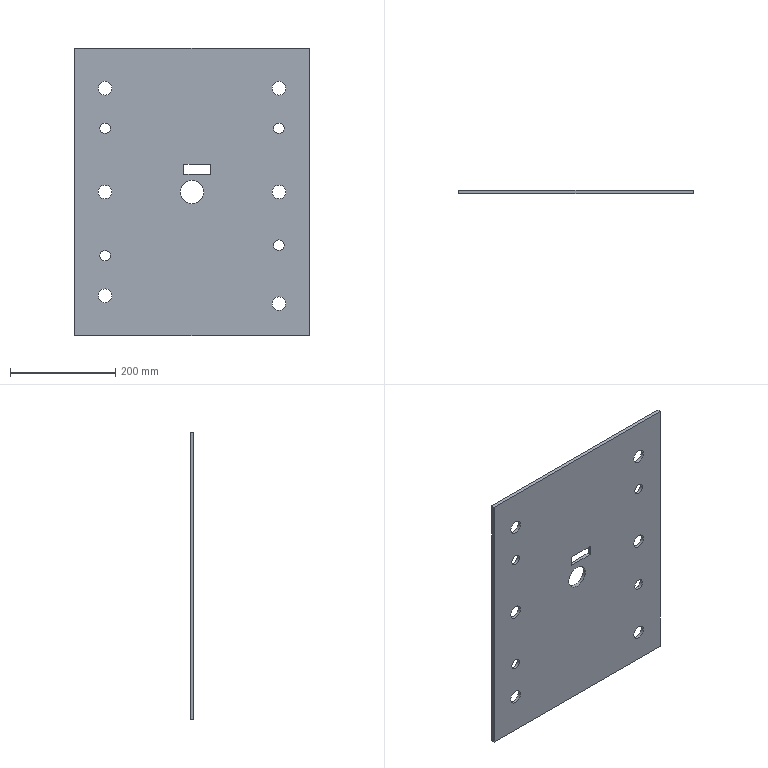Part | STEP file | INSULT-PLATE_id454_x_t | 1 solid | 21 faces | box 446 x 6 x 546 mm | volume 1419506 mm3 | cylinder 11 | plane 10 | commonest cylinder face diameters 26 x6 20 x4 44 x1
STEP:
#1=CARTESIAN_POINT('',(35.5,-296.5,34.));
#2=VERTEX_POINT('',#1);
#3=CARTESIAN_POINT('',(-15.5,-296.5,34.));
#4=VERTEX_POINT('',#3);
#5=CARTESIAN_POINT('',(-15.5,-296.5,34.));
#6=DIRECTION('',(-1.,0.,0.));
#7=VECTOR('',#6,1.);
#8=LINE('',#5,#7);
#9=EDGE_CURVE('',#2,#4,#8,.T.);
#10=ORIENTED_EDGE('',*,*,#9,.T.);
#11=CARTESIAN_POINT('',(-15.5,-296.5,53.));
#12=VERTEX_POINT('',#11);
#13=CARTESIAN_POINT('',(-15.5,-296.5,53.));
#14=DIRECTION('',(0.,0.,1.));
#15=VECTOR('',#14,1.);
#16=LINE('',#13,#15);
#17=EDGE_CURVE('',#4,#12,#16,.T.);
#18=ORIENTED_EDGE('',*,*,#17,.T.);
#19=CARTESIAN_POINT('',(35.5,-296.5,53.));
#20=VERTEX_POINT('',#19);
#21=CARTESIAN_POINT('',(35.5,-296.5,53.));
#22=DIRECTION('',(1.,0.,0.));
#23=VECTOR('',#22,1.);
#24=LINE('',#21,#23);
#25=EDGE_CURVE('',#12,#20,#24,.T.);
#26=ORIENTED_EDGE('',*,*,#25,.T.);
#27=CARTESIAN_POINT('',(35.5,-296.5,34.));
#28=DIRECTION('',(0.,0.,-1.));
#29=VECTOR('',#28,1.);
#30=LINE('',#27,#29);
#31=EDGE_CURVE('',#20,#2,#30,.T.);
#32=ORIENTED_EDGE('',*,*,#31,.T.);
#33=EDGE_LOOP('',(#10,#18,#26,#32));
#34=FACE_BOUND('',#33,.T.);
#35=CARTESIAN_POINT('',(165.,-296.5,-225.));
#36=VERTEX_POINT('',#35);
#37=CARTESIAN_POINT('',(165.,-296.5,-212.));
#38=DIRECTION('',(0.,1.,0.));
#39=DIRECTION('',(0.,0.,-1.));
#40=AXIS2_PLACEMENT_3D('',#37,#38,#39);
#41=CIRCLE('',#40,13.);
#42=EDGE_CURVE('',#36,#36,#41,.T.);
#43=ORIENTED_EDGE('',*,*,#42,.T.);
#44=EDGE_LOOP('',(#43));
#45=FACE_BOUND('',#44,.T.);
#46=CARTESIAN_POINT('',(165.,-296.5,-111.));
#47=VERTEX_POINT('',#46);
#48=CARTESIAN_POINT('',(165.,-296.5,-101.));
#49=DIRECTION('',(0.,1.,0.));
#50=DIRECTION('',(0.,0.,-1.));
#51=AXIS2_PLACEMENT_3D('',#48,#49,#50);
#52=CIRCLE('',#51,10.);
#53=EDGE_CURVE('',#47,#47,#52,.T.);
#54=ORIENTED_EDGE('',*,*,#53,.T.);
#55=EDGE_LOOP('',(#54));
#56=FACE_BOUND('',#55,.T.);
#57=CARTESIAN_POINT('',(165.,-296.5,-13.));
#58=VERTEX_POINT('',#57);
#59=CARTESIAN_POINT('',(165.,-296.5,0.));
#60=DIRECTION('',(0.,1.,0.));
#61=DIRECTION('',(0.,0.,-1.));
#62=AXIS2_PLACEMENT_3D('',#59,#60,#61);
#63=CIRCLE('',#62,13.);
#64=EDGE_CURVE('',#58,#58,#63,.T.);
#65=ORIENTED_EDGE('',*,*,#64,.T.);
#66=EDGE_LOOP('',(#65));
#67=FACE_BOUND('',#66,.T.);
#68=CARTESIAN_POINT('',(165.,-296.5,111.));
#69=VERTEX_POINT('',#68);
#70=CARTESIAN_POINT('',(165.,-296.5,121.));
#71=DIRECTION('',(0.,1.,0.));
#72=DIRECTION('',(0.,0.,-1.));
#73=AXIS2_PLACEMENT_3D('',#70,#71,#72);
#74=CIRCLE('',#73,10.);
#75=EDGE_CURVE('',#69,#69,#74,.T.);
#76=ORIENTED_EDGE('',*,*,#75,.T.);
#77=EDGE_LOOP('',(#76));
#78=FACE_BOUND('',#77,.T.);
#79=CARTESIAN_POINT('',(165.,-296.5,184.));
#80=VERTEX_POINT('',#79);
#81=CARTESIAN_POINT('',(165.,-296.5,197.));
#82=DIRECTION('',(0.,1.,0.));
#83=DIRECTION('',(0.,0.,-1.));
#84=AXIS2_PLACEMENT_3D('',#81,#82,#83);
#85=CIRCLE('',#84,13.);
#86=EDGE_CURVE('',#80,#80,#85,.T.);
#87=ORIENTED_EDGE('',*,*,#86,.T.);
#88=EDGE_LOOP('',(#87));
#89=FACE_BOUND('',#88,.T.);
#90=CARTESIAN_POINT('',(-165.,-296.5,184.));
#91=VERTEX_POINT('',#90);
#92=CARTESIAN_POINT('',(-165.,-296.5,197.));
#93=DIRECTION('',(0.,1.,0.));
#94=DIRECTION('',(0.,0.,-1.));
#95=AXIS2_PLACEMENT_3D('',#92,#93,#94);
#96=CIRCLE('',#95,13.);
#97=EDGE_CURVE('',#91,#91,#96,.T.);
#98=ORIENTED_EDGE('',*,*,#97,.T.);
#99=EDGE_LOOP('',(#98));
#100=FACE_BOUND('',#99,.T.);
#101=CARTESIAN_POINT('',(-165.,-296.5,111.));
#102=VERTEX_POINT('',#101);
#103=CARTESIAN_POINT('',(-165.,-296.5,121.));
#104=DIRECTION('',(0.,1.,0.));
#105=DIRECTION('',(0.,0.,-1.));
#106=AXIS2_PLACEMENT_3D('',#103,#104,#105);
#107=CIRCLE('',#106,10.);
#108=EDGE_CURVE('',#102,#102,#107,.T.);
#109=ORIENTED_EDGE('',*,*,#108,.T.);
#110=EDGE_LOOP('',(#109));
#111=FACE_BOUND('',#110,.T.);
#112=CARTESIAN_POINT('',(-165.,-296.5,-13.));
#113=VERTEX_POINT('',#112);
#114=CARTESIAN_POINT('',(-165.,-296.5,0.));
#115=DIRECTION('',(0.,1.,0.));
#116=DIRECTION('',(0.,0.,-1.));
#117=AXIS2_PLACEMENT_3D('',#114,#115,#116);
#118=CIRCLE('',#117,13.);
#119=EDGE_CURVE('',#113,#113,#118,.T.);
#120=ORIENTED_EDGE('',*,*,#119,.T.);
#121=EDGE_LOOP('',(#120));
#122=FACE_BOUND('',#121,.T.);
#123=CARTESIAN_POINT('',(-165.,-296.5,-131.));
#124=VERTEX_POINT('',#123);
#125=CARTESIAN_POINT('',(-165.,-296.5,-121.));
#126=DIRECTION('',(0.,1.,0.));
#127=DIRECTION('',(0.,0.,-1.));
#128=AXIS2_PLACEMENT_3D('',#125,#126,#127);
#129=CIRCLE('',#128,10.);
#130=EDGE_CURVE('',#124,#124,#129,.T.);
#131=ORIENTED_EDGE('',*,*,#130,.T.);
#132=EDGE_LOOP('',(#131));
#133=FACE_BOUND('',#132,.T.);
#134=CARTESIAN_POINT('',(-165.,-296.5,-210.));
#135=VERTEX_POINT('',#134);
#136=CARTESIAN_POINT('',(-165.,-296.5,-197.));
#137=DIRECTION('',(0.,1.,0.));
#138=DIRECTION('',(0.,0.,-1.));
#139=AXIS2_PLACEMENT_3D('',#136,#137,#138);
#140=CIRCLE('',#139,13.);
#141=EDGE_CURVE('',#135,#135,#140,.T.);
#142=ORIENTED_EDGE('',*,*,#141,.T.);
#143=EDGE_LOOP('',(#142));
#144=FACE_BOUND('',#143,.T.);
#145=CARTESIAN_POINT('',(0.,-296.5,-22.));
#146=VERTEX_POINT('',#145);
#147=CARTESIAN_POINT('',(0.,-296.5,0.));
#148=DIRECTION('',(0.,1.,0.));
#149=DIRECTION('',(0.,0.,-1.));
#150=AXIS2_PLACEMENT_3D('',#147,#148,#149);
#151=CIRCLE('',#150,22.);
#152=EDGE_CURVE('',#146,#146,#151,.T.);
#153=ORIENTED_EDGE('',*,*,#152,.T.);
#154=EDGE_LOOP('',(#153));
#155=FACE_BOUND('',#154,.T.);
#156=CARTESIAN_POINT('',(-223.,-296.5,273.));
#157=VERTEX_POINT('',#156);
#158=CARTESIAN_POINT('',(223.,-296.5,273.));
#159=VERTEX_POINT('',#158);
#160=CARTESIAN_POINT('',(223.,-296.5,273.));
#161=DIRECTION('',(1.,0.,0.));
#162=VECTOR('',#161,1.);
#163=LINE('',#160,#162);
#164=EDGE_CURVE('',#157,#159,#163,.T.);
#165=ORIENTED_EDGE('',*,*,#164,.F.);
#166=CARTESIAN_POINT('',(-223.,-296.5,-273.));
#167=VERTEX_POINT('',#166);
#168=CARTESIAN_POINT('',(-223.,-296.5,273.));
#169=DIRECTION('',(0.,0.,1.));
#170=VECTOR('',#169,1.);
#171=LINE('',#168,#170);
#172=EDGE_CURVE('',#167,#157,#171,.T.);
#173=ORIENTED_EDGE('',*,*,#172,.F.);
#174=CARTESIAN_POINT('',(223.,-296.5,-273.));
#175=VERTEX_POINT('',#174);
#176=CARTESIAN_POINT('',(-223.,-296.5,-273.));
#177=DIRECTION('',(-1.,0.,0.));
#178=VECTOR('',#177,1.);
#179=LINE('',#176,#178);
#180=EDGE_CURVE('',#175,#167,#179,.T.);
#181=ORIENTED_EDGE('',*,*,#180,.F.);
#182=CARTESIAN_POINT('',(223.,-296.5,-273.));
#183=DIRECTION('',(0.,0.,-1.));
#184=VECTOR('',#183,1.);
#185=LINE('',#182,#184);
#186=EDGE_CURVE('',#159,#175,#185,.T.);
#187=ORIENTED_EDGE('',*,*,#186,.F.);
#188=EDGE_LOOP('',(#165,#173,#181,#187));
#189=FACE_BOUND('',#188,.T.);
#190=CARTESIAN_POINT('',(225.,-296.5,275.));
#191=DIRECTION('',(0.,-1.,0.));
#192=DIRECTION('',(0.,0.,-1.));
#193=AXIS2_PLACEMENT_3D('',#190,#191,#192);
#194=PLANE('',#193);
#195=ADVANCED_FACE('',(#34,#45,#56,#67,#78,#89,#100,#111,#122,#133,#144,#155,#189),#194,.T.);
#196=CARTESIAN_POINT('',(-223.,-290.5,273.));
#197=VERTEX_POINT('',#196);
#198=CARTESIAN_POINT('',(-223.,-290.5,273.));
#199=DIRECTION('',(0.,-1.,0.));
#200=VECTOR('',#199,1.);
#201=LINE('',#198,#200);
#202=EDGE_CURVE('',#197,#157,#201,.T.);
#203=ORIENTED_EDGE('',*,*,#202,.F.);
#204=CARTESIAN_POINT('',(-223.,-290.5,-273.));
#205=VERTEX_POINT('',#204);
#206=CARTESIAN_POINT('',(-223.,-290.5,275.));
#207=DIRECTION('',(0.,0.,-1.));
#208=VECTOR('',#207,1.);
#209=LINE('',#206,#208);
#210=EDGE_CURVE('',#197,#205,#209,.T.);
#211=ORIENTED_EDGE('',*,*,#210,.T.);
#212=CARTESIAN_POINT('',(-223.,-290.5,-273.));
#213=DIRECTION('',(0.,1.,0.));
#214=VECTOR('',#213,1.);
#215=LINE('',#212,#214);
#216=EDGE_CURVE('',#167,#205,#215,.T.);
#217=ORIENTED_EDGE('',*,*,#216,.F.);
#218=ORIENTED_EDGE('',*,*,#172,.T.);
#219=EDGE_LOOP('',(#203,#211,#217,#218));
#220=FACE_OUTER_BOUND('',#219,.T.);
#221=CARTESIAN_POINT('',(-223.,-290.5,273.));
#222=DIRECTION('',(-1.,0.,0.));
#223=DIRECTION('',(0.,0.,1.));
#224=AXIS2_PLACEMENT_3D('',#221,#222,#223);
#225=PLANE('',#224);
#226=ADVANCED_FACE('',(#220),#225,.T.);
#227=ORIENTED_EDGE('',*,*,#216,.T.);
#228=CARTESIAN_POINT('',(223.,-290.5,-273.));
#229=VERTEX_POINT('',#228);
#230=CARTESIAN_POINT('',(225.,-290.5,-273.));
#231=DIRECTION('',(1.,0.,0.));
#232=VECTOR('',#231,1.);
#233=LINE('',#230,#232);
#234=EDGE_CURVE('',#205,#229,#233,.T.);
#235=ORIENTED_EDGE('',*,*,#234,.T.);
#236=CARTESIAN_POINT('',(223.,-290.5,-273.));
#237=DIRECTION('',(0.,1.,0.));
#238=VECTOR('',#237,1.);
#239=LINE('',#236,#238);
#240=EDGE_CURVE('',#175,#229,#239,.T.);
#241=ORIENTED_EDGE('',*,*,#240,.F.);
#242=ORIENTED_EDGE('',*,*,#180,.T.);
#243=EDGE_LOOP('',(#227,#235,#241,#242));
#244=FACE_OUTER_BOUND('',#243,.T.);
#245=CARTESIAN_POINT('',(-223.,-290.5,-273.));
#246=DIRECTION('',(0.,0.,-1.));
#247=DIRECTION('',(-1.,0.,0.));
#248=AXIS2_PLACEMENT_3D('',#245,#246,#247);
#249=PLANE('',#248);
#250=ADVANCED_FACE('',(#244),#249,.T.);
#251=ORIENTED_EDGE('',*,*,#240,.T.);
#252=CARTESIAN_POINT('',(223.,-290.5,273.));
#253=VERTEX_POINT('',#252);
#254=CARTESIAN_POINT('',(223.,-290.5,275.));
#255=DIRECTION('',(0.,0.,1.));
#256=VECTOR('',#255,1.);
#257=LINE('',#254,#256);
#258=EDGE_CURVE('',#229,#253,#257,.T.);
#259=ORIENTED_EDGE('',*,*,#258,.T.);
#260=CARTESIAN_POINT('',(223.,-290.5,273.));
#261=DIRECTION('',(0.,1.,0.));
#262=VECTOR('',#261,1.);
#263=LINE('',#260,#262);
#264=EDGE_CURVE('',#159,#253,#263,.T.);
#265=ORIENTED_EDGE('',*,*,#264,.F.);
#266=ORIENTED_EDGE('',*,*,#186,.T.);
#267=EDGE_LOOP('',(#251,#259,#265,#266));
#268=FACE_OUTER_BOUND('',#267,.T.);
#269=CARTESIAN_POINT('',(223.,-290.5,-273.));
#270=DIRECTION('',(1.,0.,0.));
#271=DIRECTION('',(0.,0.,-1.));
#272=AXIS2_PLACEMENT_3D('',#269,#270,#271);
#273=PLANE('',#272);
#274=ADVANCED_FACE('',(#268),#273,.T.);
#275=ORIENTED_EDGE('',*,*,#264,.T.);
#276=CARTESIAN_POINT('',(225.,-290.5,273.));
#277=DIRECTION('',(-1.,0.,0.));
#278=VECTOR('',#277,1.);
#279=LINE('',#276,#278);
#280=EDGE_CURVE('',#253,#197,#279,.T.);
#281=ORIENTED_EDGE('',*,*,#280,.T.);
#282=ORIENTED_EDGE('',*,*,#202,.T.);
#283=ORIENTED_EDGE('',*,*,#164,.T.);
#284=EDGE_LOOP('',(#275,#281,#282,#283));
#285=FACE_OUTER_BOUND('',#284,.T.);
#286=CARTESIAN_POINT('',(223.,-290.5,273.));
#287=DIRECTION('',(0.,0.,1.));
#288=DIRECTION('',(1.,0.,0.));
#289=AXIS2_PLACEMENT_3D('',#286,#287,#288);
#290=PLANE('',#289);
#291=ADVANCED_FACE('',(#285),#290,.T.);
#292=ORIENTED_EDGE('',*,*,#152,.F.);
#293=EDGE_LOOP('',(#292));
#294=FACE_BOUND('',#293,.T.);
#295=CARTESIAN_POINT('',(0.,-290.5,-22.));
#296=VERTEX_POINT('',#295);
#297=CARTESIAN_POINT('',(0.,-290.5,0.));
#298=DIRECTION('',(0.,1.,0.));
#299=DIRECTION('',(0.,0.,-1.));
#300=AXIS2_PLACEMENT_3D('',#297,#298,#299);
#301=CIRCLE('',#300,22.);
#302=EDGE_CURVE('',#296,#296,#301,.T.);
#303=ORIENTED_EDGE('',*,*,#302,.T.);
#304=EDGE_LOOP('',(#303));
#305=FACE_BOUND('',#304,.T.);
#306=CARTESIAN_POINT('',(0.,-290.5,0.));
#307=DIRECTION('',(0.,-1.,0.));
#308=DIRECTION('',(0.,0.,-1.));
#309=AXIS2_PLACEMENT_3D('',#306,#307,#308);
#310=CYLINDRICAL_SURFACE('',#309,22.);
#311=ADVANCED_FACE('',(#294,#305),#310,.F.);
#312=ORIENTED_EDGE('',*,*,#141,.F.);
#313=EDGE_LOOP('',(#312));
#314=FACE_BOUND('',#313,.T.);
#315=CARTESIAN_POINT('',(-165.,-290.5,-210.));
#316=VERTEX_POINT('',#315);
#317=CARTESIAN_POINT('',(-165.,-290.5,-197.));
#318=DIRECTION('',(0.,1.,0.));
#319=DIRECTION('',(0.,0.,-1.));
#320=AXIS2_PLACEMENT_3D('',#317,#318,#319);
#321=CIRCLE('',#320,13.);
#322=EDGE_CURVE('',#316,#316,#321,.T.);
#323=ORIENTED_EDGE('',*,*,#322,.T.);
#324=EDGE_LOOP('',(#323));
#325=FACE_BOUND('',#324,.T.);
#326=CARTESIAN_POINT('',(-165.,-296.5,-197.));
#327=DIRECTION('',(0.,-1.,0.));
#328=DIRECTION('',(0.,0.,-1.));
#329=AXIS2_PLACEMENT_3D('',#326,#327,#328);
#330=CYLINDRICAL_SURFACE('',#329,13.);
#331=ADVANCED_FACE('',(#314,#325),#330,.F.);
#332=ORIENTED_EDGE('',*,*,#130,.F.);
#333=EDGE_LOOP('',(#332));
#334=FACE_BOUND('',#333,.T.);
#335=CARTESIAN_POINT('',(-165.,-290.5,-131.));
#336=VERTEX_POINT('',#335);
#337=CARTESIAN_POINT('',(-165.,-290.5,-121.));
#338=DIRECTION('',(0.,1.,0.));
#339=DIRECTION('',(0.,0.,-1.));
#340=AXIS2_PLACEMENT_3D('',#337,#338,#339);
#341=CIRCLE('',#340,10.);
#342=EDGE_CURVE('',#336,#336,#341,.T.);
#343=ORIENTED_EDGE('',*,*,#342,.T.);
#344=EDGE_LOOP('',(#343));
#345=FACE_BOUND('',#344,.T.);
#346=CARTESIAN_POINT('',(-165.,-296.5,-121.));
#347=DIRECTION('',(0.,-1.,0.));
#348=DIRECTION('',(0.,0.,-1.));
#349=AXIS2_PLACEMENT_3D('',#346,#347,#348);
#350=CYLINDRICAL_SURFACE('',#349,10.);
#351=ADVANCED_FACE('',(#334,#345),#350,.F.);
#352=ORIENTED_EDGE('',*,*,#119,.F.);
#353=EDGE_LOOP('',(#352));
#354=FACE_BOUND('',#353,.T.);
#355=CARTESIAN_POINT('',(-165.,-290.5,-13.));
#356=VERTEX_POINT('',#355);
#357=CARTESIAN_POINT('',(-165.,-290.5,0.));
#358=DIRECTION('',(0.,1.,0.));
#359=DIRECTION('',(0.,0.,-1.));
#360=AXIS2_PLACEMENT_3D('',#357,#358,#359);
#361=CIRCLE('',#360,13.);
#362=EDGE_CURVE('',#356,#356,#361,.T.);
#363=ORIENTED_EDGE('',*,*,#362,.T.);
#364=EDGE_LOOP('',(#363));
#365=FACE_BOUND('',#364,.T.);
#366=CARTESIAN_POINT('',(-165.,-296.5,0.));
#367=DIRECTION('',(0.,-1.,0.));
#368=DIRECTION('',(0.,0.,-1.));
#369=AXIS2_PLACEMENT_3D('',#366,#367,#368);
#370=CYLINDRICAL_SURFACE('',#369,13.);
#371=ADVANCED_FACE('',(#354,#365),#370,.F.);
#372=ORIENTED_EDGE('',*,*,#108,.F.);
#373=EDGE_LOOP('',(#372));
#374=FACE_BOUND('',#373,.T.);
#375=CARTESIAN_POINT('',(-165.,-290.5,111.));
#376=VERTEX_POINT('',#375);
#377=CARTESIAN_POINT('',(-165.,-290.5,121.));
#378=DIRECTION('',(0.,1.,0.));
#379=DIRECTION('',(0.,0.,-1.));
#380=AXIS2_PLACEMENT_3D('',#377,#378,#379);
#381=CIRCLE('',#380,10.);
#382=EDGE_CURVE('',#376,#376,#381,.T.);
#383=ORIENTED_EDGE('',*,*,#382,.T.);
#384=EDGE_LOOP('',(#383));
#385=FACE_BOUND('',#384,.T.);
#386=CARTESIAN_POINT('',(-165.,-296.5,121.));
#387=DIRECTION('',(0.,-1.,0.));
#388=DIRECTION('',(0.,0.,-1.));
#389=AXIS2_PLACEMENT_3D('',#386,#387,#388);
#390=CYLINDRICAL_SURFACE('',#389,10.);
#391=ADVANCED_FACE('',(#374,#385),#390,.F.);
#392=ORIENTED_EDGE('',*,*,#97,.F.);
#393=EDGE_LOOP('',(#392));
#394=FACE_BOUND('',#393,.T.);
#395=CARTESIAN_POINT('',(-165.,-290.5,184.));
#396=VERTEX_POINT('',#395);
#397=CARTESIAN_POINT('',(-165.,-290.5,197.));
#398=DIRECTION('',(0.,1.,0.));
#399=DIRECTION('',(0.,0.,-1.));
#400=AXIS2_PLACEMENT_3D('',#397,#398,#399);
#401=CIRCLE('',#400,13.);
#402=EDGE_CURVE('',#396,#396,#401,.T.);
#403=ORIENTED_EDGE('',*,*,#402,.T.);
#404=EDGE_LOOP('',(#403));
#405=FACE_BOUND('',#404,.T.);
#406=CARTESIAN_POINT('',(-165.,-296.5,197.));
#407=DIRECTION('',(0.,-1.,0.));
#408=DIRECTION('',(0.,0.,-1.));
#409=AXIS2_PLACEMENT_3D('',#406,#407,#408);
#410=CYLINDRICAL_SURFACE('',#409,13.);
#411=ADVANCED_FACE('',(#394,#405),#410,.F.);
#412=ORIENTED_EDGE('',*,*,#86,.F.);
#413=EDGE_LOOP('',(#412));
#414=FACE_BOUND('',#413,.T.);
#415=CARTESIAN_POINT('',(165.,-290.5,184.));
#416=VERTEX_POINT('',#415);
#417=CARTESIAN_POINT('',(165.,-290.5,197.));
#418=DIRECTION('',(0.,1.,0.));
#419=DIRECTION('',(0.,0.,-1.));
#420=AXIS2_PLACEMENT_3D('',#417,#418,#419);
#421=CIRCLE('',#420,13.);
#422=EDGE_CURVE('',#416,#416,#421,.T.);
#423=ORIENTED_EDGE('',*,*,#422,.T.);
#424=EDGE_LOOP('',(#423));
#425=FACE_BOUND('',#424,.T.);
#426=CARTESIAN_POINT('',(165.,-296.5,197.));
#427=DIRECTION('',(0.,-1.,0.));
#428=DIRECTION('',(0.,0.,-1.));
#429=AXIS2_PLACEMENT_3D('',#426,#427,#428);
#430=CYLINDRICAL_SURFACE('',#429,13.);
#431=ADVANCED_FACE('',(#414,#425),#430,.F.);
#432=ORIENTED_EDGE('',*,*,#75,.F.);
#433=EDGE_LOOP('',(#432));
#434=FACE_BOUND('',#433,.T.);
#435=CARTESIAN_POINT('',(165.,-290.5,111.));
#436=VERTEX_POINT('',#435);
#437=CARTESIAN_POINT('',(165.,-290.5,121.));
#438=DIRECTION('',(0.,1.,0.));
#439=DIRECTION('',(0.,0.,-1.));
#440=AXIS2_PLACEMENT_3D('',#437,#438,#439);
#441=CIRCLE('',#440,10.);
#442=EDGE_CURVE('',#436,#436,#441,.T.);
#443=ORIENTED_EDGE('',*,*,#442,.T.);
#444=EDGE_LOOP('',(#443));
#445=FACE_BOUND('',#444,.T.);
#446=CARTESIAN_POINT('',(165.,-296.5,121.));
#447=DIRECTION('',(0.,-1.,0.));
#448=DIRECTION('',(0.,0.,-1.));
#449=AXIS2_PLACEMENT_3D('',#446,#447,#448);
#450=CYLINDRICAL_SURFACE('',#449,10.);
#451=ADVANCED_FACE('',(#434,#445),#450,.F.);
#452=ORIENTED_EDGE('',*,*,#64,.F.);
#453=EDGE_LOOP('',(#452));
#454=FACE_BOUND('',#453,.T.);
#455=CARTESIAN_POINT('',(165.,-290.5,-13.));
#456=VERTEX_POINT('',#455);
#457=CARTESIAN_POINT('',(165.,-290.5,0.));
#458=DIRECTION('',(0.,1.,0.));
#459=DIRECTION('',(0.,0.,-1.));
#460=AXIS2_PLACEMENT_3D('',#457,#458,#459);
#461=CIRCLE('',#460,13.);
#462=EDGE_CURVE('',#456,#456,#461,.T.);
#463=ORIENTED_EDGE('',*,*,#462,.T.);
#464=EDGE_LOOP('',(#463));
#465=FACE_BOUND('',#464,.T.);
#466=CARTESIAN_POINT('',(165.,-296.5,0.));
#467=DIRECTION('',(0.,-1.,0.));
#468=DIRECTION('',(0.,0.,-1.));
#469=AXIS2_PLACEMENT_3D('',#466,#467,#468);
#470=CYLINDRICAL_SURFACE('',#469,13.);
#471=ADVANCED_FACE('',(#454,#465),#470,.F.);
#472=ORIENTED_EDGE('',*,*,#53,.F.);
#473=EDGE_LOOP('',(#472));
#474=FACE_BOUND('',#473,.T.);
#475=CARTESIAN_POINT('',(165.,-290.5,-111.));
#476=VERTEX_POINT('',#475);
#477=CARTESIAN_POINT('',(165.,-290.5,-101.));
#478=DIRECTION('',(0.,1.,0.));
#479=DIRECTION('',(0.,0.,-1.));
#480=AXIS2_PLACEMENT_3D('',#477,#478,#479);
#481=CIRCLE('',#480,10.);
#482=EDGE_CURVE('',#476,#476,#481,.T.);
#483=ORIENTED_EDGE('',*,*,#482,.T.);
#484=EDGE_LOOP('',(#483));
#485=FACE_BOUND('',#484,.T.);
#486=CARTESIAN_POINT('',(165.,-296.5,-101.));
#487=DIRECTION('',(0.,-1.,0.));
#488=DIRECTION('',(0.,0.,-1.));
#489=AXIS2_PLACEMENT_3D('',#486,#487,#488);
#490=CYLINDRICAL_SURFACE('',#489,10.);
#491=ADVANCED_FACE('',(#474,#485),#490,.F.);
#492=ORIENTED_EDGE('',*,*,#42,.F.);
#493=EDGE_LOOP('',(#492));
#494=FACE_BOUND('',#493,.T.);
#495=CARTESIAN_POINT('',(165.,-290.5,-225.));
#496=VERTEX_POINT('',#495);
#497=CARTESIAN_POINT('',(165.,-290.5,-212.));
#498=DIRECTION('',(0.,1.,0.));
#499=DIRECTION('',(0.,0.,-1.));
#500=AXIS2_PLACEMENT_3D('',#497,#498,#499);
#501=CIRCLE('',#500,13.);
#502=EDGE_CURVE('',#496,#496,#501,.T.);
#503=ORIENTED_EDGE('',*,*,#502,.T.);
#504=EDGE_LOOP('',(#503));
#505=FACE_BOUND('',#504,.T.);
#506=CARTESIAN_POINT('',(165.,-296.5,-212.));
#507=DIRECTION('',(0.,-1.,0.));
#508=DIRECTION('',(0.,0.,-1.));
#509=AXIS2_PLACEMENT_3D('',#506,#507,#508);
#510=CYLINDRICAL_SURFACE('',#509,13.);
#511=ADVANCED_FACE('',(#494,#505),#510,.F.);
#512=ORIENTED_EDGE('',*,*,#17,.F.);
#513=CARTESIAN_POINT('',(-15.5,-290.5,34.));
#514=VERTEX_POINT('',#513);
#515=CARTESIAN_POINT('',(-15.5,-296.5,34.));
#516=DIRECTION('',(0.,1.,0.));
#517=VECTOR('',#516,1.);
#518=LINE('',#515,#517);
#519=EDGE_CURVE('',#4,#514,#518,.T.);
#520=ORIENTED_EDGE('',*,*,#519,.T.);
#521=CARTESIAN_POINT('',(-15.5,-290.5,53.));
#522=VERTEX_POINT('',#521);
#523=CARTESIAN_POINT('',(-15.5,-290.5,275.));
#524=DIRECTION('',(0.,0.,1.));
#525=VECTOR('',#524,1.);
#526=LINE('',#523,#525);
#527=EDGE_CURVE('',#514,#522,#526,.T.);
#528=ORIENTED_EDGE('',*,*,#527,.T.);
#529=CARTESIAN_POINT('',(-15.5,-296.5,53.));
#530=DIRECTION('',(0.,-1.,0.));
#531=VECTOR('',#530,1.);
#532=LINE('',#529,#531);
#533=EDGE_CURVE('',#522,#12,#532,.T.);
#534=ORIENTED_EDGE('',*,*,#533,.T.);
#535=EDGE_LOOP('',(#512,#520,#528,#534));
#536=FACE_OUTER_BOUND('',#535,.T.);
#537=CARTESIAN_POINT('',(-15.5,-296.5,53.));
#538=DIRECTION('',(-1.,0.,0.));
#539=DIRECTION('',(0.,0.,1.));
#540=AXIS2_PLACEMENT_3D('',#537,#538,#539);
#541=PLANE('',#540);
#542=ADVANCED_FACE('',(#536),#541,.F.);
#543=ORIENTED_EDGE('',*,*,#25,.F.);
#544=ORIENTED_EDGE('',*,*,#533,.F.);
#545=CARTESIAN_POINT('',(35.5,-290.5,53.));
#546=VERTEX_POINT('',#545);
#547=CARTESIAN_POINT('',(225.,-290.5,53.));
#548=DIRECTION('',(1.,0.,0.));
#549=VECTOR('',#548,1.);
#550=LINE('',#547,#549);
#551=EDGE_CURVE('',#522,#546,#550,.T.);
#552=ORIENTED_EDGE('',*,*,#551,.T.);
#553=CARTESIAN_POINT('',(35.5,-296.5,53.));
#554=DIRECTION('',(0.,-1.,0.));
#555=VECTOR('',#554,1.);
#556=LINE('',#553,#555);
#557=EDGE_CURVE('',#546,#20,#556,.T.);
#558=ORIENTED_EDGE('',*,*,#557,.T.);
#559=EDGE_LOOP('',(#543,#544,#552,#558));
#560=FACE_OUTER_BOUND('',#559,.T.);
#561=CARTESIAN_POINT('',(35.5,-296.5,53.));
#562=DIRECTION('',(0.,0.,1.));
#563=DIRECTION('',(1.,0.,0.));
#564=AXIS2_PLACEMENT_3D('',#561,#562,#563);
#565=PLANE('',#564);
#566=ADVANCED_FACE('',(#560),#565,.F.);
#567=ORIENTED_EDGE('',*,*,#31,.F.);
#568=ORIENTED_EDGE('',*,*,#557,.F.);
#569=CARTESIAN_POINT('',(35.5,-290.5,34.));
#570=VERTEX_POINT('',#569);
#571=CARTESIAN_POINT('',(35.5,-290.5,275.));
#572=DIRECTION('',(0.,0.,-1.));
#573=VECTOR('',#572,1.);
#574=LINE('',#571,#573);
#575=EDGE_CURVE('',#546,#570,#574,.T.);
#576=ORIENTED_EDGE('',*,*,#575,.T.);
#577=CARTESIAN_POINT('',(35.5,-296.5,34.));
#578=DIRECTION('',(0.,-1.,0.));
#579=VECTOR('',#578,1.);
#580=LINE('',#577,#579);
#581=EDGE_CURVE('',#570,#2,#580,.T.);
#582=ORIENTED_EDGE('',*,*,#581,.T.);
#583=EDGE_LOOP('',(#567,#568,#576,#582));
#584=FACE_OUTER_BOUND('',#583,.T.);
#585=CARTESIAN_POINT('',(35.5,-296.5,34.));
#586=DIRECTION('',(1.,0.,0.));
#587=DIRECTION('',(0.,0.,-1.));
#588=AXIS2_PLACEMENT_3D('',#585,#586,#587);
#589=PLANE('',#588);
#590=ADVANCED_FACE('',(#584),#589,.F.);
#591=ORIENTED_EDGE('',*,*,#9,.F.);
#592=ORIENTED_EDGE('',*,*,#581,.F.);
#593=CARTESIAN_POINT('',(225.,-290.5,34.));
#594=DIRECTION('',(-1.,0.,0.));
#595=VECTOR('',#594,1.);
#596=LINE('',#593,#595);
#597=EDGE_CURVE('',#570,#514,#596,.T.);
#598=ORIENTED_EDGE('',*,*,#597,.T.);
#599=ORIENTED_EDGE('',*,*,#519,.F.);
#600=EDGE_LOOP('',(#591,#592,#598,#599));
#601=FACE_OUTER_BOUND('',#600,.T.);
#602=CARTESIAN_POINT('',(-15.5,-296.5,34.));
#603=DIRECTION('',(0.,0.,-1.));
#604=DIRECTION('',(-1.,0.,0.));
#605=AXIS2_PLACEMENT_3D('',#602,#603,#604);
#606=PLANE('',#605);
#607=ADVANCED_FACE('',(#601),#606,.F.);
#608=ORIENTED_EDGE('',*,*,#575,.F.);
#609=ORIENTED_EDGE('',*,*,#551,.F.);
#610=ORIENTED_EDGE('',*,*,#527,.F.);
#611=ORIENTED_EDGE('',*,*,#597,.F.);
#612=EDGE_LOOP('',(#608,#609,#610,#611));
#613=FACE_BOUND('',#612,.T.);
#614=ORIENTED_EDGE('',*,*,#502,.F.);
#615=EDGE_LOOP('',(#614));
#616=FACE_BOUND('',#615,.T.);
#617=ORIENTED_EDGE('',*,*,#482,.F.);
#618=EDGE_LOOP('',(#617));
#619=FACE_BOUND('',#618,.T.);
#620=ORIENTED_EDGE('',*,*,#462,.F.);
#621=EDGE_LOOP('',(#620));
#622=FACE_BOUND('',#621,.T.);
#623=ORIENTED_EDGE('',*,*,#442,.F.);
#624=EDGE_LOOP('',(#623));
#625=FACE_BOUND('',#624,.T.);
#626=ORIENTED_EDGE('',*,*,#422,.F.);
#627=EDGE_LOOP('',(#626));
#628=FACE_BOUND('',#627,.T.);
#629=ORIENTED_EDGE('',*,*,#402,.F.);
#630=EDGE_LOOP('',(#629));
#631=FACE_BOUND('',#630,.T.);
#632=ORIENTED_EDGE('',*,*,#382,.F.);
#633=EDGE_LOOP('',(#632));
#634=FACE_BOUND('',#633,.T.);
#635=ORIENTED_EDGE('',*,*,#362,.F.);
#636=EDGE_LOOP('',(#635));
#637=FACE_BOUND('',#636,.T.);
#638=ORIENTED_EDGE('',*,*,#342,.F.);
#639=EDGE_LOOP('',(#638));
#640=FACE_BOUND('',#639,.T.);
#641=ORIENTED_EDGE('',*,*,#322,.F.);
#642=EDGE_LOOP('',(#641));
#643=FACE_BOUND('',#642,.T.);
#644=ORIENTED_EDGE('',*,*,#302,.F.);
#645=EDGE_LOOP('',(#644));
#646=FACE_BOUND('',#645,.T.);
#647=ORIENTED_EDGE('',*,*,#258,.F.);
#648=ORIENTED_EDGE('',*,*,#234,.F.);
#649=ORIENTED_EDGE('',*,*,#210,.F.);
#650=ORIENTED_EDGE('',*,*,#280,.F.);
#651=EDGE_LOOP('',(#647,#648,#649,#650));
#652=FACE_BOUND('',#651,.T.);
#653=CARTESIAN_POINT('',(225.,-290.5,275.));
#654=DIRECTION('',(0.,-1.,0.));
#655=DIRECTION('',(0.,0.,-1.));
#656=AXIS2_PLACEMENT_3D('',#653,#654,#655);
#657=PLANE('',#656);
#658=ADVANCED_FACE('',(#613,#616,#619,#622,#625,#628,#631,#634,#637,#640,#643,#646,#652),#657,.F.);
#659=CLOSED_SHELL('',(#195,#226,#250,#274,#291,#311,#331,#351,#371,#391,#411,#431,#451,#471,#491,#511,#542,#566,#590,#607,#658));
#660=MANIFOLD_SOLID_BREP('',#659);
#661=(LENGTH_UNIT()NAMED_UNIT(*)SI_UNIT(.MILLI.,.METRE.));
#662=UNCERTAINTY_MEASURE_WITH_UNIT(LENGTH_MEASURE(0.00002),#661,'','');
#663=(NAMED_UNIT(*)PLANE_ANGLE_UNIT()SI_UNIT($,.RADIAN.));
#664=PLANE_ANGLE_MEASURE_WITH_UNIT(PLANE_ANGLE_MEASURE(0.01745),#663);
#665=DIMENSIONAL_EXPONENTS(0.,0.,0.,0.,0.,0.,0.);
#666=(CONVERSION_BASED_UNIT('DEGREE',#664)NAMED_UNIT(#665)PLANE_ANGLE_UNIT());
#667=(NAMED_UNIT(*)SI_UNIT($,.STERADIAN.)SOLID_ANGLE_UNIT());
#668=(GEOMETRIC_REPRESENTATION_CONTEXT(3)GLOBAL_UNCERTAINTY_ASSIGNED_CONTEXT((#662))GLOBAL_UNIT_ASSIGNED_CONTEXT((#661,#666,#667))REPRESENTATION_CONTEXT('',''));
#669=ADVANCED_BREP_SHAPE_REPRESENTATION('',(#660),#668);